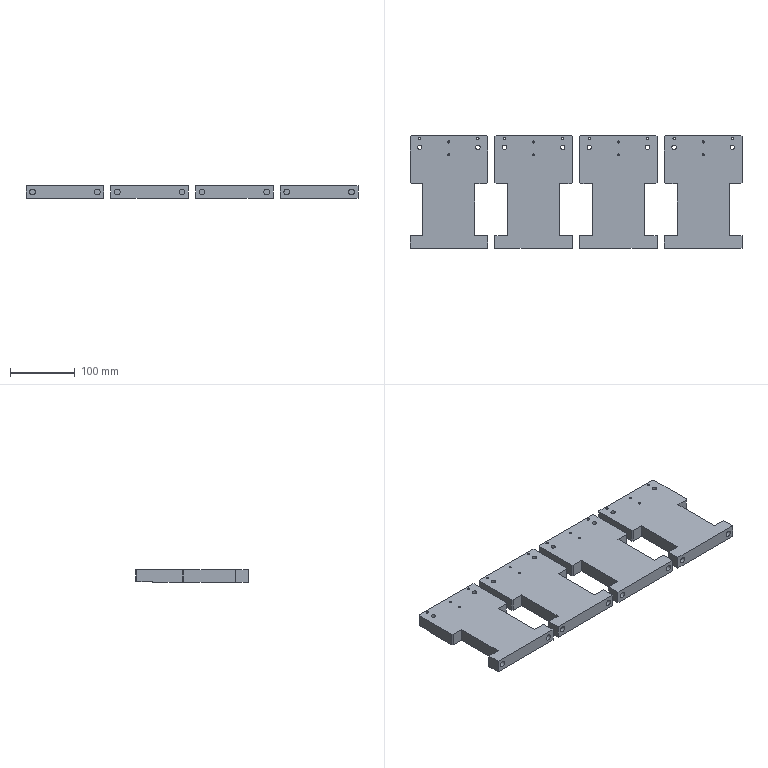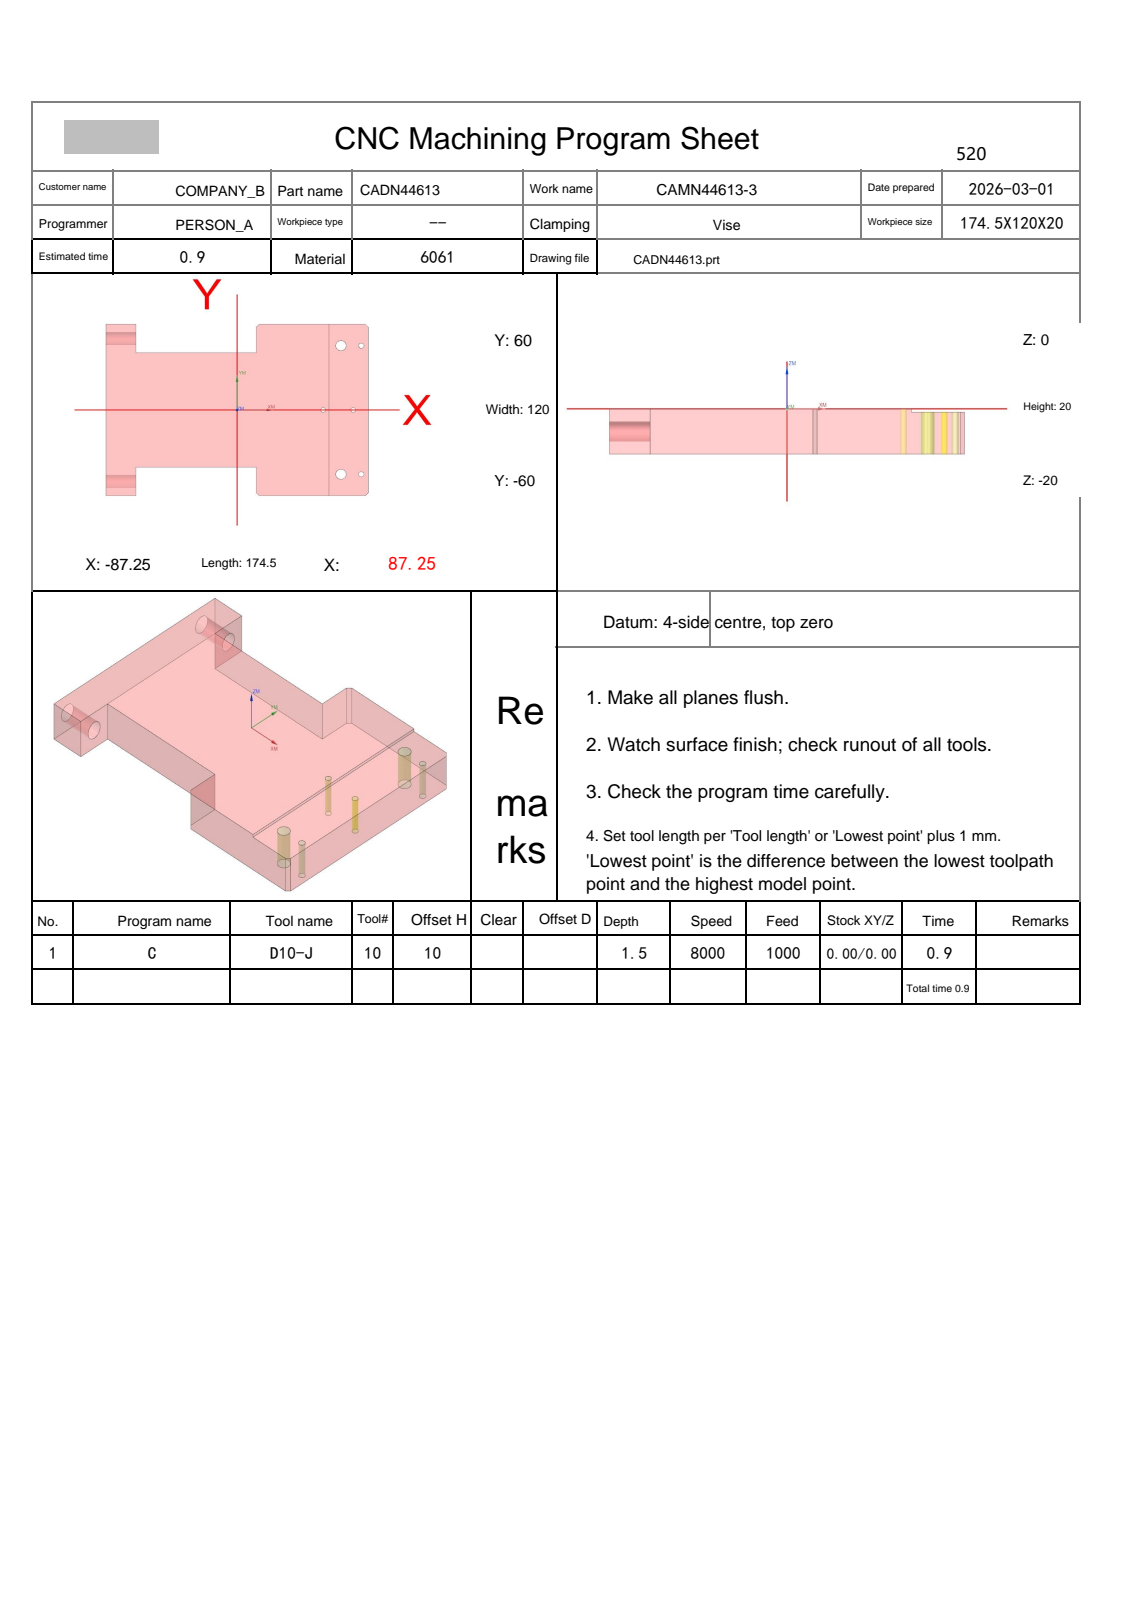NC program | NX | posted by the shop | part box 513 x 174.5 x 20 mm
Whole program:
%
O0001
(Machine time: 1.11 MIN)
(===Total Tool:1===)
(T10=D10-J  D=10.  R=0.   D10 H10 Z=-1.5  )
G80 G90 G17 G49 G40
G91 G28 Z0
M01
N1 T10 M06
(D10-J  D=10. R=0. H=10 ce=0.40 di=0.00)
(D.N=10 MAX_Z=10.5 MIN_Z=-1.5 Time=0.91M)
G00 G90 G54 X94.25 Y2. M03 S8000
G43 H10 Z10.4
M08
Z0.0
G01 Z-1.5 F1000.
X90.25
G03 X88.25 Y0.0 I0.0 J-2.
G01 Y-58.003
G02 X87.959 Y-58.705 I-1. J.003
G01 X85.955 Y-60.709
G02 X85.253 Y-61. I-.705 J.709
G01 X67.497
G02 X66.5 Y-60.003 I.003 J1.
G01 Y60.003
G02 X67.497 Y61. I1. J-.003
G01 X85.253
G02 X85.957 Y60.707 I-.003 J-1.
G01 X87.959 Y58.705
G02 X88.25 Y58.003 I-.709 J-.705
G01 Y-2.086
G02 X87.958 Y-2.792 I-1. J.001
G01 X83.542 Y-7.208
G03 X83.25 Y-7.914 I.708 J-.707
G01 Y-55.004
G02 X82.254 Y-56. I-1. J.004
G01 X72.496
G02 X71.5 Y-55.004 I.004 J1.
G01 Y55.004
G02 X72.496 Y56. I1. J-.004
G01 X82.254
G02 X83.25 Y55.004 I-.004 J-1.
G01 Y-2.086
G02 X82.958 Y-2.792 I-1. J.001
G01 X78.542 Y-7.208
G03 X78.25 Y-7.914 I.708 J-.707
G01 Y-50.203
G02 X77.453 Y-51. I-.8 J.003
G01 X77.297
G02 X76.5 Y-50.203 I.003 J.8
G01 Y50.203
G02 X77.297 Y51. I.8 J-.003
G01 X77.453
G02 X78.25 Y50.203 I-.003 J-.8
G01 Y-5.
Y-6.
G03 X80.25 Y-8. I2. J0.0
G01 Z0.0
G00 Z10.4
G00 G90 X68.299 Y67. M03 S8000
Z10.5
Z-.5
G01 Z-1.5 F1000.
G41 D10
X68.099
G03 X66.1 Y65. I.001 J-2.
G01 Y-65.
G03 X68.099 Y-67. I2. J0.0
G01 G40 X68.299
Z-.5
G00 Z10.5
M05
M09
G91 G28 Z0.0
G91 G28 Y0.0
M30
%